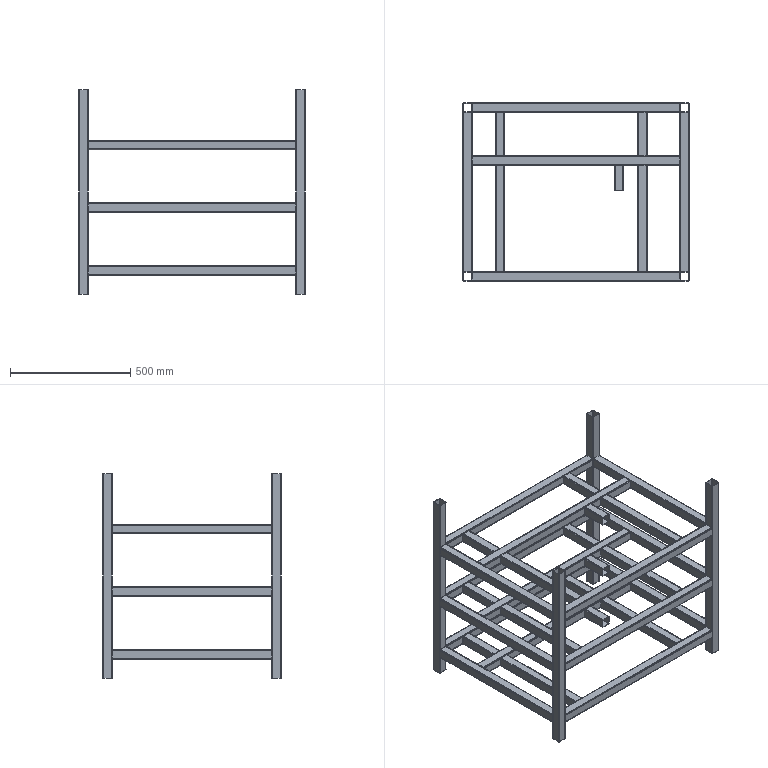Part | SolidWorks | features 3DProfileFeature 1, WeldMemberFeat 1, WeldmentFeature 1 | 34 solids | 612 faces | box 940 x 740 x 850 mm | volume 8249556 mm3 | plane 340 | cylinder 272 | commonest cylinder face diameters 2 x136 8 x136